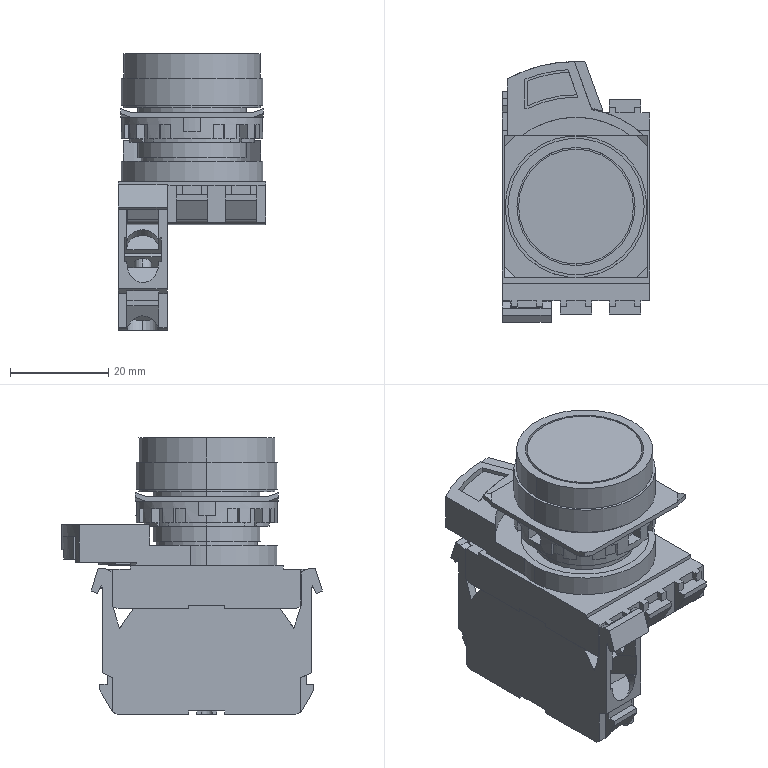Part | STEP file | A22NN_BNM_NRA_G100_NN | 5 solids | 511 faces | box 30 x 53 x 56.3 mm | volume 27846 mm3 | plane 405 | cylinder 106 | commonest cylinder face diameters 25.4 x10 27 x8 28.8 x7 4 x6 6.5 x6 20.8 x5